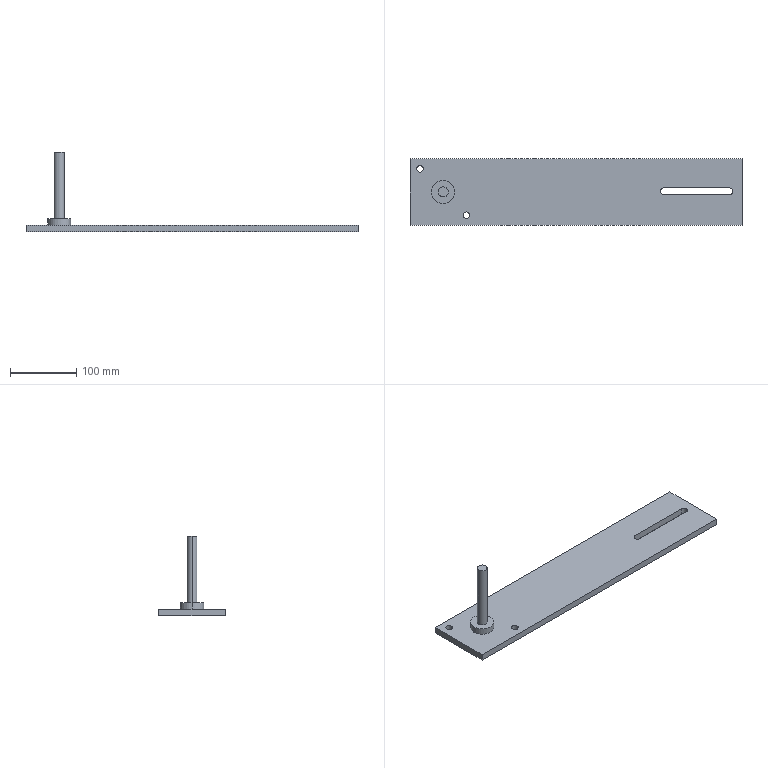Part | SolidWorks | features ICE 5, Extrusion 1 | 1 solid | 24 faces | box 500 x 100 x 120 mm | volume 514971 mm3 | cylinder 12 | plane 12 | commonest cylinder face diameters 9 x4 10 x4 15 x2 35 x2
STEP:
#1=CARTESIAN_POINT('',(-192.5,0.,20.));
#2=VERTEX_POINT('',#1);
#3=CARTESIAN_POINT('',(-207.5,0.,20.));
#4=VERTEX_POINT('',#3);
#5=CARTESIAN_POINT('',(-200.,0.,20.));
#6=DIRECTION('',(0.,0.,1.));
#7=DIRECTION('',(1.,0.,0.));
#8=AXIS2_PLACEMENT_3D('',#5,#6,#7);
#9=CIRCLE('',#8,7.5);
#10=EDGE_CURVE('',#2,#4,#9,.T.);
#11=ORIENTED_EDGE('',*,*,#10,.T.);
#12=CARTESIAN_POINT('',(-207.5,0.,120.));
#13=VERTEX_POINT('',#12);
#14=CARTESIAN_POINT('',(-207.5,0.,20.));
#15=DIRECTION('',(0.,0.,1.));
#16=VECTOR('',#15,1000.);
#17=LINE('',#14,#16);
#18=EDGE_CURVE('',#4,#13,#17,.T.);
#19=ORIENTED_EDGE('',*,*,#18,.T.);
#20=CARTESIAN_POINT('',(-192.5,0.,120.));
#21=VERTEX_POINT('',#20);
#22=CARTESIAN_POINT('',(-200.,0.,120.));
#23=DIRECTION('',(0.,0.,1.));
#24=DIRECTION('',(1.,0.,0.));
#25=AXIS2_PLACEMENT_3D('',#22,#23,#24);
#26=CIRCLE('',#25,7.5);
#27=EDGE_CURVE('',#21,#13,#26,.T.);
#28=ORIENTED_EDGE('',*,*,#27,.F.);
#29=CARTESIAN_POINT('',(-192.5,0.,20.));
#30=DIRECTION('',(0.,0.,1.));
#31=VECTOR('',#30,1000.);
#32=LINE('',#29,#31);
#33=EDGE_CURVE('',#2,#21,#32,.T.);
#34=ORIENTED_EDGE('',*,*,#33,.F.);
#35=EDGE_LOOP('',(#11,#19,#28,#34));
#36=FACE_OUTER_BOUND('',#35,.T.);
#37=CARTESIAN_POINT('',(-200.,0.,20.));
#38=DIRECTION('',(0.,0.,1.));
#39=DIRECTION('',(1.,0.,0.));
#40=AXIS2_PLACEMENT_3D('',#37,#38,#39);
#41=CYLINDRICAL_SURFACE('',#40,7.5);
#42=ADVANCED_FACE('',(#36),#41,.T.);
#43=CARTESIAN_POINT('',(-160.,-35.,0.));
#44=VERTEX_POINT('',#43);
#45=CARTESIAN_POINT('',(-170.,-35.,0.));
#46=VERTEX_POINT('',#45);
#47=CARTESIAN_POINT('',(-165.,-35.,0.));
#48=DIRECTION('',(0.,0.,-1.));
#49=DIRECTION('',(-1.,0.,0.));
#50=AXIS2_PLACEMENT_3D('',#47,#48,#49);
#51=CIRCLE('',#50,5.);
#52=EDGE_CURVE('',#44,#46,#51,.T.);
#53=ORIENTED_EDGE('',*,*,#52,.T.);
#54=CARTESIAN_POINT('',(-170.,-35.,10.));
#55=VERTEX_POINT('',#54);
#56=CARTESIAN_POINT('',(-170.,-35.,-50.));
#57=DIRECTION('',(0.,0.,1.));
#58=VECTOR('',#57,1000.);
#59=LINE('',#56,#58);
#60=EDGE_CURVE('',#46,#55,#59,.T.);
#61=ORIENTED_EDGE('',*,*,#60,.T.);
#62=CARTESIAN_POINT('',(-160.,-35.,10.));
#63=VERTEX_POINT('',#62);
#64=CARTESIAN_POINT('',(-165.,-35.,10.));
#65=DIRECTION('',(0.,0.,1.));
#66=DIRECTION('',(1.,0.,0.));
#67=AXIS2_PLACEMENT_3D('',#64,#65,#66);
#68=CIRCLE('',#67,5.);
#69=EDGE_CURVE('',#55,#63,#68,.T.);
#70=ORIENTED_EDGE('',*,*,#69,.T.);
#71=CARTESIAN_POINT('',(-160.,-35.,-50.));
#72=DIRECTION('',(0.,0.,1.));
#73=VECTOR('',#72,1000.);
#74=LINE('',#71,#73);
#75=EDGE_CURVE('',#44,#63,#74,.T.);
#76=ORIENTED_EDGE('',*,*,#75,.F.);
#77=EDGE_LOOP('',(#53,#61,#70,#76));
#78=FACE_OUTER_BOUND('',#77,.T.);
#79=CARTESIAN_POINT('',(-165.,-35.,-50.));
#80=DIRECTION('',(0.,0.,1.));
#81=DIRECTION('',(1.,0.,0.));
#82=AXIS2_PLACEMENT_3D('',#79,#80,#81);
#83=CYLINDRICAL_SURFACE('',#82,5.);
#84=ADVANCED_FACE('',(#78),#83,.F.);
#85=CARTESIAN_POINT('',(-230.,35.,0.));
#86=VERTEX_POINT('',#85);
#87=CARTESIAN_POINT('',(-240.,35.,0.));
#88=VERTEX_POINT('',#87);
#89=CARTESIAN_POINT('',(-235.,35.,0.));
#90=DIRECTION('',(0.,0.,-1.));
#91=DIRECTION('',(-1.,0.,0.));
#92=AXIS2_PLACEMENT_3D('',#89,#90,#91);
#93=CIRCLE('',#92,5.);
#94=EDGE_CURVE('',#86,#88,#93,.T.);
#95=ORIENTED_EDGE('',*,*,#94,.T.);
#96=CARTESIAN_POINT('',(-240.,35.,10.));
#97=VERTEX_POINT('',#96);
#98=CARTESIAN_POINT('',(-240.,35.,-50.));
#99=DIRECTION('',(0.,0.,1.));
#100=VECTOR('',#99,1000.);
#101=LINE('',#98,#100);
#102=EDGE_CURVE('',#88,#97,#101,.T.);
#103=ORIENTED_EDGE('',*,*,#102,.T.);
#104=CARTESIAN_POINT('',(-230.,35.,10.));
#105=VERTEX_POINT('',#104);
#106=CARTESIAN_POINT('',(-235.,35.,10.));
#107=DIRECTION('',(0.,0.,1.));
#108=DIRECTION('',(1.,0.,0.));
#109=AXIS2_PLACEMENT_3D('',#106,#107,#108);
#110=CIRCLE('',#109,5.);
#111=EDGE_CURVE('',#97,#105,#110,.T.);
#112=ORIENTED_EDGE('',*,*,#111,.T.);
#113=CARTESIAN_POINT('',(-230.,35.,-50.));
#114=DIRECTION('',(0.,0.,1.));
#115=VECTOR('',#114,1000.);
#116=LINE('',#113,#115);
#117=EDGE_CURVE('',#86,#105,#116,.T.);
#118=ORIENTED_EDGE('',*,*,#117,.F.);
#119=EDGE_LOOP('',(#95,#103,#112,#118));
#120=FACE_OUTER_BOUND('',#119,.T.);
#121=CARTESIAN_POINT('',(-235.,35.,-50.));
#122=DIRECTION('',(0.,0.,1.));
#123=DIRECTION('',(1.,0.,0.));
#124=AXIS2_PLACEMENT_3D('',#121,#122,#123);
#125=CYLINDRICAL_SURFACE('',#124,5.);
#126=ADVANCED_FACE('',(#120),#125,.F.);
#127=CARTESIAN_POINT('',(-182.5,0.,20.));
#128=VERTEX_POINT('',#127);
#129=CARTESIAN_POINT('',(-217.5,0.,20.));
#130=VERTEX_POINT('',#129);
#131=CARTESIAN_POINT('',(-200.,0.,20.));
#132=DIRECTION('',(0.,0.,1.));
#133=DIRECTION('',(1.,0.,0.));
#134=AXIS2_PLACEMENT_3D('',#131,#132,#133);
#135=CIRCLE('',#134,17.5);
#136=EDGE_CURVE('',#128,#130,#135,.T.);
#137=ORIENTED_EDGE('',*,*,#136,.F.);
#138=CARTESIAN_POINT('',(-182.5,0.,10.));
#139=VERTEX_POINT('',#138);
#140=CARTESIAN_POINT('',(-182.5,0.,70.));
#141=DIRECTION('',(0.,0.,-1.));
#142=VECTOR('',#141,1000.);
#143=LINE('',#140,#142);
#144=EDGE_CURVE('',#128,#139,#143,.T.);
#145=ORIENTED_EDGE('',*,*,#144,.T.);
#146=CARTESIAN_POINT('',(-217.5,0.,10.));
#147=VERTEX_POINT('',#146);
#148=CARTESIAN_POINT('',(-200.,0.,10.));
#149=DIRECTION('',(0.,0.,1.));
#150=DIRECTION('',(-1.,0.,0.));
#151=AXIS2_PLACEMENT_3D('',#148,#149,#150);
#152=CIRCLE('',#151,17.5);
#153=EDGE_CURVE('',#139,#147,#152,.T.);
#154=ORIENTED_EDGE('',*,*,#153,.T.);
#155=CARTESIAN_POINT('',(-217.5,0.,70.));
#156=DIRECTION('',(0.,0.,-1.));
#157=VECTOR('',#156,1000.);
#158=LINE('',#155,#157);
#159=EDGE_CURVE('',#130,#147,#158,.T.);
#160=ORIENTED_EDGE('',*,*,#159,.F.);
#161=EDGE_LOOP('',(#137,#145,#154,#160));
#162=FACE_OUTER_BOUND('',#161,.T.);
#163=CARTESIAN_POINT('',(-200.,0.,70.));
#164=DIRECTION('',(0.,0.,-1.));
#165=DIRECTION('',(-1.,0.,0.));
#166=AXIS2_PLACEMENT_3D('',#163,#164,#165);
#167=CYLINDRICAL_SURFACE('',#166,17.5);
#168=ADVANCED_FACE('',(#162),#167,.T.);
#169=ORIENTED_EDGE('',*,*,#144,.F.);
#170=CARTESIAN_POINT('',(-200.,0.,20.));
#171=DIRECTION('',(0.,0.,1.));
#172=DIRECTION('',(1.,0.,0.));
#173=AXIS2_PLACEMENT_3D('',#170,#171,#172);
#174=CIRCLE('',#173,17.5);
#175=EDGE_CURVE('',#130,#128,#174,.T.);
#176=ORIENTED_EDGE('',*,*,#175,.F.);
#177=ORIENTED_EDGE('',*,*,#159,.T.);
#178=CARTESIAN_POINT('',(-200.,0.,10.));
#179=DIRECTION('',(0.,0.,1.));
#180=DIRECTION('',(-1.,0.,0.));
#181=AXIS2_PLACEMENT_3D('',#178,#179,#180);
#182=CIRCLE('',#181,17.5);
#183=EDGE_CURVE('',#147,#139,#182,.T.);
#184=ORIENTED_EDGE('',*,*,#183,.T.);
#185=EDGE_LOOP('',(#169,#176,#177,#184));
#186=FACE_OUTER_BOUND('',#185,.T.);
#187=CARTESIAN_POINT('',(-200.,0.,70.));
#188=DIRECTION('',(0.,0.,-1.));
#189=DIRECTION('',(-1.,0.,0.));
#190=AXIS2_PLACEMENT_3D('',#187,#188,#189);
#191=CYLINDRICAL_SURFACE('',#190,17.5);
#192=ADVANCED_FACE('',(#186),#191,.T.);
#193=CARTESIAN_POINT('',(-250.,50.,10.));
#194=VERTEX_POINT('',#193);
#195=CARTESIAN_POINT('',(-250.,-50.,10.));
#196=VERTEX_POINT('',#195);
#197=CARTESIAN_POINT('',(-250.,50.,10.));
#198=DIRECTION('',(0.,-1.,0.));
#199=VECTOR('',#198,1000.);
#200=LINE('',#197,#199);
#201=EDGE_CURVE('',#194,#196,#200,.T.);
#202=ORIENTED_EDGE('',*,*,#201,.T.);
#203=CARTESIAN_POINT('',(250.,-50.,10.));
#204=VERTEX_POINT('',#203);
#205=CARTESIAN_POINT('',(250.,-50.,10.));
#206=DIRECTION('',(1.,0.,0.));
#207=VECTOR('',#206,1000.);
#208=LINE('',#205,#207);
#209=EDGE_CURVE('',#196,#204,#208,.T.);
#210=ORIENTED_EDGE('',*,*,#209,.T.);
#211=CARTESIAN_POINT('',(250.,50.,10.));
#212=VERTEX_POINT('',#211);
#213=CARTESIAN_POINT('',(250.,50.,10.));
#214=DIRECTION('',(0.,1.,0.));
#215=VECTOR('',#214,1000.);
#216=LINE('',#213,#215);
#217=EDGE_CURVE('',#204,#212,#216,.T.);
#218=ORIENTED_EDGE('',*,*,#217,.T.);
#219=CARTESIAN_POINT('',(250.,50.,10.));
#220=DIRECTION('',(-1.,0.,0.));
#221=VECTOR('',#220,1000.);
#222=LINE('',#219,#221);
#223=EDGE_CURVE('',#212,#194,#222,.T.);
#224=ORIENTED_EDGE('',*,*,#223,.T.);
#225=EDGE_LOOP('',(#202,#210,#218,#224));
#226=FACE_OUTER_BOUND('',#225,.T.);
#227=CARTESIAN_POINT('',(231.805,6.068,10.));
#228=VERTEX_POINT('',#227);
#229=CARTESIAN_POINT('',(131.558,6.068,10.));
#230=VERTEX_POINT('',#229);
#231=CARTESIAN_POINT('',(231.805,6.068,10.));
#232=DIRECTION('',(-1.,0.,0.));
#233=VECTOR('',#232,1000.);
#234=LINE('',#231,#233);
#235=EDGE_CURVE('',#228,#230,#234,.T.);
#236=ORIENTED_EDGE('',*,*,#235,.F.);
#237=CARTESIAN_POINT('',(236.305,1.568,10.));
#238=VERTEX_POINT('',#237);
#239=CARTESIAN_POINT('',(231.805,1.568,10.));
#240=DIRECTION('',(0.,0.,1.));
#241=DIRECTION('',(1.,0.,0.));
#242=AXIS2_PLACEMENT_3D('',#239,#240,#241);
#243=CIRCLE('',#242,4.5);
#244=EDGE_CURVE('',#238,#228,#243,.T.);
#245=ORIENTED_EDGE('',*,*,#244,.F.);
#246=CARTESIAN_POINT('',(236.305,0.5678,10.));
#247=VERTEX_POINT('',#246);
#248=CARTESIAN_POINT('',(236.305,0.5678,10.));
#249=DIRECTION('',(0.,1.,0.));
#250=VECTOR('',#249,1000.);
#251=LINE('',#248,#250);
#252=EDGE_CURVE('',#247,#238,#251,.T.);
#253=ORIENTED_EDGE('',*,*,#252,.F.);
#254=CARTESIAN_POINT('',(231.805,-3.932,10.));
#255=VERTEX_POINT('',#254);
#256=CARTESIAN_POINT('',(231.805,0.5678,10.));
#257=DIRECTION('',(0.,0.,1.));
#258=DIRECTION('',(1.,0.,0.));
#259=AXIS2_PLACEMENT_3D('',#256,#257,#258);
#260=CIRCLE('',#259,4.5);
#261=EDGE_CURVE('',#255,#247,#260,.T.);
#262=ORIENTED_EDGE('',*,*,#261,.F.);
#263=CARTESIAN_POINT('',(131.558,-3.932,10.));
#264=VERTEX_POINT('',#263);
#265=CARTESIAN_POINT('',(231.805,-3.932,10.));
#266=DIRECTION('',(1.,0.,0.));
#267=VECTOR('',#266,1000.);
#268=LINE('',#265,#267);
#269=EDGE_CURVE('',#264,#255,#268,.T.);
#270=ORIENTED_EDGE('',*,*,#269,.F.);
#271=CARTESIAN_POINT('',(127.058,0.5678,10.));
#272=VERTEX_POINT('',#271);
#273=CARTESIAN_POINT('',(131.558,0.5678,10.));
#274=DIRECTION('',(0.,0.,1.));
#275=DIRECTION('',(-1.,0.,0.));
#276=AXIS2_PLACEMENT_3D('',#273,#274,#275);
#277=CIRCLE('',#276,4.5);
#278=EDGE_CURVE('',#272,#264,#277,.T.);
#279=ORIENTED_EDGE('',*,*,#278,.F.);
#280=CARTESIAN_POINT('',(127.058,1.568,10.));
#281=VERTEX_POINT('',#280);
#282=CARTESIAN_POINT('',(127.058,0.5678,10.));
#283=DIRECTION('',(0.,-1.,0.));
#284=VECTOR('',#283,1000.);
#285=LINE('',#282,#284);
#286=EDGE_CURVE('',#281,#272,#285,.T.);
#287=ORIENTED_EDGE('',*,*,#286,.F.);
#288=CARTESIAN_POINT('',(131.558,1.568,10.));
#289=DIRECTION('',(0.,0.,1.));
#290=DIRECTION('',(-1.,0.,0.));
#291=AXIS2_PLACEMENT_3D('',#288,#289,#290);
#292=CIRCLE('',#291,4.5);
#293=EDGE_CURVE('',#230,#281,#292,.T.);
#294=ORIENTED_EDGE('',*,*,#293,.F.);
#295=EDGE_LOOP('',(#236,#245,#253,#262,#270,#279,#287,#294));
#296=FACE_BOUND('',#295,.T.);
#297=CARTESIAN_POINT('',(-235.,35.,10.));
#298=DIRECTION('',(0.,0.,1.));
#299=DIRECTION('',(1.,0.,0.));
#300=AXIS2_PLACEMENT_3D('',#297,#298,#299);
#301=CIRCLE('',#300,5.);
#302=EDGE_CURVE('',#105,#97,#301,.T.);
#303=ORIENTED_EDGE('',*,*,#302,.F.);
#304=ORIENTED_EDGE('',*,*,#111,.F.);
#305=EDGE_LOOP('',(#303,#304));
#306=FACE_BOUND('',#305,.T.);
#307=CARTESIAN_POINT('',(-165.,-35.,10.));
#308=DIRECTION('',(0.,0.,1.));
#309=DIRECTION('',(1.,0.,0.));
#310=AXIS2_PLACEMENT_3D('',#307,#308,#309);
#311=CIRCLE('',#310,5.);
#312=EDGE_CURVE('',#63,#55,#311,.T.);
#313=ORIENTED_EDGE('',*,*,#312,.F.);
#314=ORIENTED_EDGE('',*,*,#69,.F.);
#315=EDGE_LOOP('',(#313,#314));
#316=FACE_BOUND('',#315,.T.);
#317=ORIENTED_EDGE('',*,*,#183,.F.);
#318=ORIENTED_EDGE('',*,*,#153,.F.);
#319=EDGE_LOOP('',(#317,#318));
#320=FACE_BOUND('',#319,.T.);
#321=CARTESIAN_POINT('',(-250.,-50.,10.));
#322=DIRECTION('',(0.,0.,-1.));
#323=DIRECTION('',(-1.,0.,0.));
#324=AXIS2_PLACEMENT_3D('',#321,#322,#323);
#325=PLANE('',#324);
#326=ADVANCED_FACE('',(#226,#296,#306,#316,#320),#325,.F.);
#327=CARTESIAN_POINT('',(-250.,50.,0.));
#328=VERTEX_POINT('',#327);
#329=CARTESIAN_POINT('',(-250.,-50.,0.));
#330=VERTEX_POINT('',#329);
#331=CARTESIAN_POINT('',(-250.,50.,0.));
#332=DIRECTION('',(0.,-1.,0.));
#333=VECTOR('',#332,1000.);
#334=LINE('',#331,#333);
#335=EDGE_CURVE('',#328,#330,#334,.T.);
#336=ORIENTED_EDGE('',*,*,#335,.T.);
#337=CARTESIAN_POINT('',(-250.,-50.,10.));
#338=DIRECTION('',(0.,0.,-1.));
#339=VECTOR('',#338,1000.);
#340=LINE('',#337,#339);
#341=EDGE_CURVE('',#196,#330,#340,.T.);
#342=ORIENTED_EDGE('',*,*,#341,.F.);
#343=ORIENTED_EDGE('',*,*,#201,.F.);
#344=CARTESIAN_POINT('',(-250.,50.,10.));
#345=DIRECTION('',(0.,0.,-1.));
#346=VECTOR('',#345,1000.);
#347=LINE('',#344,#346);
#348=EDGE_CURVE('',#194,#328,#347,.T.);
#349=ORIENTED_EDGE('',*,*,#348,.T.);
#350=EDGE_LOOP('',(#336,#342,#343,#349));
#351=FACE_OUTER_BOUND('',#350,.T.);
#352=CARTESIAN_POINT('',(-250.,50.,10.));
#353=DIRECTION('',(1.,0.,0.));
#354=DIRECTION('',(0.,0.,-1.));
#355=AXIS2_PLACEMENT_3D('',#352,#353,#354);
#356=PLANE('',#355);
#357=ADVANCED_FACE('',(#351),#356,.F.);
#358=CARTESIAN_POINT('',(250.,-50.,0.));
#359=VERTEX_POINT('',#358);
#360=CARTESIAN_POINT('',(250.,-50.,0.));
#361=DIRECTION('',(1.,0.,0.));
#362=VECTOR('',#361,1000.);
#363=LINE('',#360,#362);
#364=EDGE_CURVE('',#330,#359,#363,.T.);
#365=ORIENTED_EDGE('',*,*,#364,.T.);
#366=CARTESIAN_POINT('',(250.,-50.,10.));
#367=DIRECTION('',(0.,0.,-1.));
#368=VECTOR('',#367,1000.);
#369=LINE('',#366,#368);
#370=EDGE_CURVE('',#204,#359,#369,.T.);
#371=ORIENTED_EDGE('',*,*,#370,.F.);
#372=ORIENTED_EDGE('',*,*,#209,.F.);
#373=ORIENTED_EDGE('',*,*,#341,.T.);
#374=EDGE_LOOP('',(#365,#371,#372,#373));
#375=FACE_OUTER_BOUND('',#374,.T.);
#376=CARTESIAN_POINT('',(250.,-50.,10.));
#377=DIRECTION('',(0.,1.,0.));
#378=DIRECTION('',(-1.,0.,0.));
#379=AXIS2_PLACEMENT_3D('',#376,#377,#378);
#380=PLANE('',#379);
#381=ADVANCED_FACE('',(#375),#380,.F.);
#382=CARTESIAN_POINT('',(250.,50.,0.));
#383=VERTEX_POINT('',#382);
#384=CARTESIAN_POINT('',(250.,50.,0.));
#385=DIRECTION('',(0.,1.,0.));
#386=VECTOR('',#385,1000.);
#387=LINE('',#384,#386);
#388=EDGE_CURVE('',#359,#383,#387,.T.);
#389=ORIENTED_EDGE('',*,*,#388,.T.);
#390=CARTESIAN_POINT('',(250.,50.,10.));
#391=DIRECTION('',(0.,0.,-1.));
#392=VECTOR('',#391,1000.);
#393=LINE('',#390,#392);
#394=EDGE_CURVE('',#212,#383,#393,.T.);
#395=ORIENTED_EDGE('',*,*,#394,.F.);
#396=ORIENTED_EDGE('',*,*,#217,.F.);
#397=ORIENTED_EDGE('',*,*,#370,.T.);
#398=EDGE_LOOP('',(#389,#395,#396,#397));
#399=FACE_OUTER_BOUND('',#398,.T.);
#400=CARTESIAN_POINT('',(250.,50.,10.));
#401=DIRECTION('',(-1.,0.,0.));
#402=DIRECTION('',(0.,0.,1.));
#403=AXIS2_PLACEMENT_3D('',#400,#401,#402);
#404=PLANE('',#403);
#405=ADVANCED_FACE('',(#399),#404,.F.);
#406=CARTESIAN_POINT('',(250.,50.,0.));
#407=DIRECTION('',(-1.,0.,0.));
#408=VECTOR('',#407,1000.);
#409=LINE('',#406,#408);
#410=EDGE_CURVE('',#383,#328,#409,.T.);
#411=ORIENTED_EDGE('',*,*,#410,.T.);
#412=ORIENTED_EDGE('',*,*,#348,.F.);
#413=ORIENTED_EDGE('',*,*,#223,.F.);
#414=ORIENTED_EDGE('',*,*,#394,.T.);
#415=EDGE_LOOP('',(#411,#412,#413,#414));
#416=FACE_OUTER_BOUND('',#415,.T.);
#417=CARTESIAN_POINT('',(250.,50.,10.));
#418=DIRECTION('',(0.,-1.,0.));
#419=DIRECTION('',(1.,0.,0.));
#420=AXIS2_PLACEMENT_3D('',#417,#418,#419);
#421=PLANE('',#420);
#422=ADVANCED_FACE('',(#416),#421,.F.);
#423=ORIENTED_EDGE('',*,*,#52,.F.);
#424=CARTESIAN_POINT('',(-165.,-35.,0.));
#425=DIRECTION('',(0.,0.,-1.));
#426=DIRECTION('',(-1.,0.,0.));
#427=AXIS2_PLACEMENT_3D('',#424,#425,#426);
#428=CIRCLE('',#427,5.);
#429=EDGE_CURVE('',#46,#44,#428,.T.);
#430=ORIENTED_EDGE('',*,*,#429,.F.);
#431=EDGE_LOOP('',(#423,#430));
#432=FACE_BOUND('',#431,.T.);
#433=ORIENTED_EDGE('',*,*,#94,.F.);
#434=CARTESIAN_POINT('',(-235.,35.,0.));
#435=DIRECTION('',(0.,0.,-1.));
#436=DIRECTION('',(-1.,0.,0.));
#437=AXIS2_PLACEMENT_3D('',#434,#435,#436);
#438=CIRCLE('',#437,5.);
#439=EDGE_CURVE('',#88,#86,#438,.T.);
#440=ORIENTED_EDGE('',*,*,#439,.F.);
#441=EDGE_LOOP('',(#433,#440));
#442=FACE_BOUND('',#441,.T.);
#443=CARTESIAN_POINT('',(231.805,6.068,0.));
#444=VERTEX_POINT('',#443);
#445=CARTESIAN_POINT('',(236.305,1.568,0.));
#446=VERTEX_POINT('',#445);
#447=CARTESIAN_POINT('',(231.805,1.568,0.));
#448=DIRECTION('',(0.,0.,-1.));
#449=DIRECTION('',(-1.,0.,0.));
#450=AXIS2_PLACEMENT_3D('',#447,#448,#449);
#451=CIRCLE('',#450,4.5);
#452=EDGE_CURVE('',#444,#446,#451,.T.);
#453=ORIENTED_EDGE('',*,*,#452,.F.);
#454=CARTESIAN_POINT('',(131.558,6.068,0.));
#455=VERTEX_POINT('',#454);
#456=CARTESIAN_POINT('',(-250.,6.068,0.));
#457=DIRECTION('',(1.,0.,0.));
#458=VECTOR('',#457,1000.);
#459=LINE('',#456,#458);
#460=EDGE_CURVE('',#455,#444,#459,.T.);
#461=ORIENTED_EDGE('',*,*,#460,.F.);
#462=CARTESIAN_POINT('',(127.058,1.568,0.));
#463=VERTEX_POINT('',#462);
#464=CARTESIAN_POINT('',(131.558,1.568,0.));
#465=DIRECTION('',(0.,0.,-1.));
#466=DIRECTION('',(-1.,0.,0.));
#467=AXIS2_PLACEMENT_3D('',#464,#465,#466);
#468=CIRCLE('',#467,4.5);
#469=EDGE_CURVE('',#463,#455,#468,.T.);
#470=ORIENTED_EDGE('',*,*,#469,.F.);
#471=CARTESIAN_POINT('',(127.058,0.5678,0.));
#472=VERTEX_POINT('',#471);
#473=CARTESIAN_POINT('',(127.058,-50.,0.));
#474=DIRECTION('',(0.,1.,0.));
#475=VECTOR('',#474,1000.);
#476=LINE('',#473,#475);
#477=EDGE_CURVE('',#472,#463,#476,.T.);
#478=ORIENTED_EDGE('',*,*,#477,.F.);
#479=CARTESIAN_POINT('',(131.558,-3.932,0.));
#480=VERTEX_POINT('',#479);
#481=CARTESIAN_POINT('',(131.558,0.5678,0.));
#482=DIRECTION('',(0.,0.,-1.));
#483=DIRECTION('',(-1.,0.,0.));
#484=AXIS2_PLACEMENT_3D('',#481,#482,#483);
#485=CIRCLE('',#484,4.5);
#486=EDGE_CURVE('',#480,#472,#485,.T.);
#487=ORIENTED_EDGE('',*,*,#486,.F.);
#488=CARTESIAN_POINT('',(231.805,-3.932,0.));
#489=VERTEX_POINT('',#488);
#490=CARTESIAN_POINT('',(-250.,-3.932,0.));
#491=DIRECTION('',(-1.,0.,0.));
#492=VECTOR('',#491,1000.);
#493=LINE('',#490,#492);
#494=EDGE_CURVE('',#489,#480,#493,.T.);
#495=ORIENTED_EDGE('',*,*,#494,.F.);
#496=CARTESIAN_POINT('',(236.305,0.5678,0.));
#497=VERTEX_POINT('',#496);
#498=CARTESIAN_POINT('',(231.805,0.5678,0.));
#499=DIRECTION('',(0.,0.,-1.));
#500=DIRECTION('',(-1.,0.,0.));
#501=AXIS2_PLACEMENT_3D('',#498,#499,#500);
#502=CIRCLE('',#501,4.5);
#503=EDGE_CURVE('',#497,#489,#502,.T.);
#504=ORIENTED_EDGE('',*,*,#503,.F.);
#505=CARTESIAN_POINT('',(236.305,-50.,0.));
#506=DIRECTION('',(0.,-1.,0.));
#507=VECTOR('',#506,1000.);
#508=LINE('',#505,#507);
#509=EDGE_CURVE('',#446,#497,#508,.T.);
#510=ORIENTED_EDGE('',*,*,#509,.F.);
#511=EDGE_LOOP('',(#453,#461,#470,#478,#487,#495,#504,#510));
#512=FACE_BOUND('',#511,.T.);
#513=ORIENTED_EDGE('',*,*,#335,.F.);
#514=ORIENTED_EDGE('',*,*,#410,.F.);
#515=ORIENTED_EDGE('',*,*,#388,.F.);
#516=ORIENTED_EDGE('',*,*,#364,.F.);
#517=EDGE_LOOP('',(#513,#514,#515,#516));
#518=FACE_OUTER_BOUND('',#517,.T.);
#519=CARTESIAN_POINT('',(-250.,-50.,0.));
#520=DIRECTION('',(0.,0.,-1.));
#521=DIRECTION('',(-1.,0.,0.));
#522=AXIS2_PLACEMENT_3D('',#519,#520,#521);
#523=PLANE('',#522);
#524=ADVANCED_FACE('',(#432,#442,#512,#518),#523,.T.);
#525=ORIENTED_EDGE('',*,*,#452,.T.);
#526=CARTESIAN_POINT('',(236.305,1.568,-50.));
#527=DIRECTION('',(0.,0.,1.));
#528=VECTOR('',#527,1000.);
#529=LINE('',#526,#528);
#530=EDGE_CURVE('',#446,#238,#529,.T.);
#531=ORIENTED_EDGE('',*,*,#530,.T.);
#532=ORIENTED_EDGE('',*,*,#244,.T.);
#533=CARTESIAN_POINT('',(231.805,6.068,-50.));
#534=DIRECTION('',(0.,0.,1.));
#535=VECTOR('',#534,1000.);
#536=LINE('',#533,#535);
#537=EDGE_CURVE('',#444,#228,#536,.T.);
#538=ORIENTED_EDGE('',*,*,#537,.F.);
#539=EDGE_LOOP('',(#525,#531,#532,#538));
#540=FACE_OUTER_BOUND('',#539,.T.);
#541=CARTESIAN_POINT('',(231.805,1.568,-50.));
#542=DIRECTION('',(0.,0.,1.));
#543=DIRECTION('',(1.,0.,0.));
#544=AXIS2_PLACEMENT_3D('',#541,#542,#543);
#545=CYLINDRICAL_SURFACE('',#544,4.5);
#546=ADVANCED_FACE('',(#540),#545,.F.);
#547=ORIENTED_EDGE('',*,*,#509,.T.);
#548=CARTESIAN_POINT('',(236.305,0.5678,-50.));
#549=DIRECTION('',(0.,0.,1.));
#550=VECTOR('',#549,1000.);
#551=LINE('',#548,#550);
#552=EDGE_CURVE('',#497,#247,#551,.T.);
#553=ORIENTED_EDGE('',*,*,#552,.T.);
#554=ORIENTED_EDGE('',*,*,#252,.T.);
#555=ORIENTED_EDGE('',*,*,#530,.F.);
#556=EDGE_LOOP('',(#547,#553,#554,#555));
#557=FACE_OUTER_BOUND('',#556,.T.);
#558=CARTESIAN_POINT('',(236.305,0.5678,-50.));
#559=DIRECTION('',(1.,0.,0.));
#560=DIRECTION('',(0.,0.,-1.));
#561=AXIS2_PLACEMENT_3D('',#558,#559,#560);
#562=PLANE('',#561);
#563=ADVANCED_FACE('',(#557),#562,.F.);
#564=ORIENTED_EDGE('',*,*,#503,.T.);
#565=CARTESIAN_POINT('',(231.805,-3.932,-50.));
#566=DIRECTION('',(0.,0.,1.));
#567=VECTOR('',#566,1000.);
#568=LINE('',#565,#567);
#569=EDGE_CURVE('',#489,#255,#568,.T.);
#570=ORIENTED_EDGE('',*,*,#569,.T.);
#571=ORIENTED_EDGE('',*,*,#261,.T.);
#572=ORIENTED_EDGE('',*,*,#552,.F.);
#573=EDGE_LOOP('',(#564,#570,#571,#572));
#574=FACE_OUTER_BOUND('',#573,.T.);
#575=CARTESIAN_POINT('',(231.805,0.5678,-50.));
#576=DIRECTION('',(0.,0.,1.));
#577=DIRECTION('',(1.,0.,0.));
#578=AXIS2_PLACEMENT_3D('',#575,#576,#577);
#579=CYLINDRICAL_SURFACE('',#578,4.5);
#580=ADVANCED_FACE('',(#574),#579,.F.);
#581=ORIENTED_EDGE('',*,*,#494,.T.);
#582=CARTESIAN_POINT('',(131.558,-3.932,-50.));
#583=DIRECTION('',(0.,0.,1.));
#584=VECTOR('',#583,1000.);
#585=LINE('',#582,#584);
#586=EDGE_CURVE('',#480,#264,#585,.T.);
#587=ORIENTED_EDGE('',*,*,#586,.T.);
#588=ORIENTED_EDGE('',*,*,#269,.T.);
#589=ORIENTED_EDGE('',*,*,#569,.F.);
#590=EDGE_LOOP('',(#581,#587,#588,#589));
#591=FACE_OUTER_BOUND('',#590,.T.);
#592=CARTESIAN_POINT('',(231.805,-3.932,-50.));
#593=DIRECTION('',(0.,-1.,0.));
#594=DIRECTION('',(1.,0.,0.));
#595=AXIS2_PLACEMENT_3D('',#592,#593,#594);
#596=PLANE('',#595);
#597=ADVANCED_FACE('',(#591),#596,.F.);
#598=ORIENTED_EDGE('',*,*,#486,.T.);
#599=CARTESIAN_POINT('',(127.058,0.5678,-50.));
#600=DIRECTION('',(0.,0.,1.));
#601=VECTOR('',#600,1000.);
#602=LINE('',#599,#601);
#603=EDGE_CURVE('',#472,#272,#602,.T.);
#604=ORIENTED_EDGE('',*,*,#603,.T.);
#605=ORIENTED_EDGE('',*,*,#278,.T.);
#606=ORIENTED_EDGE('',*,*,#586,.F.);
#607=EDGE_LOOP('',(#598,#604,#605,#606));
#608=FACE_OUTER_BOUND('',#607,.T.);
#609=CARTESIAN_POINT('',(131.558,0.5678,-50.));
#610=DIRECTION('',(0.,0.,1.));
#611=DIRECTION('',(1.,0.,0.));
#612=AXIS2_PLACEMENT_3D('',#609,#610,#611);
#613=CYLINDRICAL_SURFACE('',#612,4.5);
#614=ADVANCED_FACE('',(#608),#613,.F.);
#615=ORIENTED_EDGE('',*,*,#477,.T.);
#616=CARTESIAN_POINT('',(127.058,1.568,-50.));
#617=DIRECTION('',(0.,0.,1.));
#618=VECTOR('',#617,1000.);
#619=LINE('',#616,#618);
#620=EDGE_CURVE('',#463,#281,#619,.T.);
#621=ORIENTED_EDGE('',*,*,#620,.T.);
#622=ORIENTED_EDGE('',*,*,#286,.T.);
#623=ORIENTED_EDGE('',*,*,#603,.F.);
#624=EDGE_LOOP('',(#615,#621,#622,#623));
#625=FACE_OUTER_BOUND('',#624,.T.);
#626=CARTESIAN_POINT('',(127.058,0.5678,-50.));
#627=DIRECTION('',(-1.,0.,0.));
#628=DIRECTION('',(0.,0.,1.));
#629=AXIS2_PLACEMENT_3D('',#626,#627,#628);
#630=PLANE('',#629);
#631=ADVANCED_FACE('',(#625),#630,.F.);
#632=ORIENTED_EDGE('',*,*,#469,.T.);
#633=CARTESIAN_POINT('',(131.558,6.068,-50.));
#634=DIRECTION('',(0.,0.,1.));
#635=VECTOR('',#634,1000.);
#636=LINE('',#633,#635);
#637=EDGE_CURVE('',#455,#230,#636,.T.);
#638=ORIENTED_EDGE('',*,*,#637,.T.);
#639=ORIENTED_EDGE('',*,*,#293,.T.);
#640=ORIENTED_EDGE('',*,*,#620,.F.);
#641=EDGE_LOOP('',(#632,#638,#639,#640));
#642=FACE_OUTER_BOUND('',#641,.T.);
#643=CARTESIAN_POINT('',(131.558,1.568,-50.));
#644=DIRECTION('',(0.,0.,1.));
#645=DIRECTION('',(1.,0.,0.));
#646=AXIS2_PLACEMENT_3D('',#643,#644,#645);
#647=CYLINDRICAL_SURFACE('',#646,4.5);
#648=ADVANCED_FACE('',(#642),#647,.F.);
#649=ORIENTED_EDGE('',*,*,#460,.T.);
#650=ORIENTED_EDGE('',*,*,#537,.T.);
#651=ORIENTED_EDGE('',*,*,#235,.T.);
#652=ORIENTED_EDGE('',*,*,#637,.F.);
#653=EDGE_LOOP('',(#649,#650,#651,#652));
#654=FACE_OUTER_BOUND('',#653,.T.);
#655=CARTESIAN_POINT('',(231.805,6.068,-50.));
#656=DIRECTION('',(0.,1.,0.));
#657=DIRECTION('',(-1.,0.,0.));
#658=AXIS2_PLACEMENT_3D('',#655,#656,#657);
#659=PLANE('',#658);
#660=ADVANCED_FACE('',(#654),#659,.F.);
#661=ORIENTED_EDGE('',*,*,#102,.F.);
#662=ORIENTED_EDGE('',*,*,#439,.T.);
#663=ORIENTED_EDGE('',*,*,#117,.T.);
#664=ORIENTED_EDGE('',*,*,#302,.T.);
#665=EDGE_LOOP('',(#661,#662,#663,#664));
#666=FACE_OUTER_BOUND('',#665,.T.);
#667=CARTESIAN_POINT('',(-235.,35.,-50.));
#668=DIRECTION('',(0.,0.,1.));
#669=DIRECTION('',(1.,0.,0.));
#670=AXIS2_PLACEMENT_3D('',#667,#668,#669);
#671=CYLINDRICAL_SURFACE('',#670,5.);
#672=ADVANCED_FACE('',(#666),#671,.F.);
#673=ORIENTED_EDGE('',*,*,#60,.F.);
#674=ORIENTED_EDGE('',*,*,#429,.T.);
#675=ORIENTED_EDGE('',*,*,#75,.T.);
#676=ORIENTED_EDGE('',*,*,#312,.T.);
#677=EDGE_LOOP('',(#673,#674,#675,#676));
#678=FACE_OUTER_BOUND('',#677,.T.);
#679=CARTESIAN_POINT('',(-165.,-35.,-50.));
#680=DIRECTION('',(0.,0.,1.));
#681=DIRECTION('',(1.,0.,0.));
#682=AXIS2_PLACEMENT_3D('',#679,#680,#681);
#683=CYLINDRICAL_SURFACE('',#682,5.);
#684=ADVANCED_FACE('',(#678),#683,.F.);
#685=ORIENTED_EDGE('',*,*,#10,.F.);
#686=CARTESIAN_POINT('',(-200.,0.,20.));
#687=DIRECTION('',(0.,0.,1.));
#688=DIRECTION('',(1.,0.,0.));
#689=AXIS2_PLACEMENT_3D('',#686,#687,#688);
#690=CIRCLE('',#689,7.5);
#691=EDGE_CURVE('',#4,#2,#690,.T.);
#692=ORIENTED_EDGE('',*,*,#691,.F.);
#693=EDGE_LOOP('',(#685,#692));
#694=FACE_BOUND('',#693,.T.);
#695=ORIENTED_EDGE('',*,*,#175,.T.);
#696=ORIENTED_EDGE('',*,*,#136,.T.);
#697=EDGE_LOOP('',(#695,#696));
#698=FACE_OUTER_BOUND('',#697,.T.);
#699=CARTESIAN_POINT('',(-200.,0.,20.));
#700=DIRECTION('',(0.,0.,1.));
#701=DIRECTION('',(1.,0.,0.));
#702=AXIS2_PLACEMENT_3D('',#699,#700,#701);
#703=PLANE('',#702);
#704=ADVANCED_FACE('',(#694,#698),#703,.T.);
#705=ORIENTED_EDGE('',*,*,#18,.F.);
#706=ORIENTED_EDGE('',*,*,#691,.T.);
#707=ORIENTED_EDGE('',*,*,#33,.T.);
#708=CARTESIAN_POINT('',(-200.,0.,120.));
#709=DIRECTION('',(0.,0.,1.));
#710=DIRECTION('',(1.,0.,0.));
#711=AXIS2_PLACEMENT_3D('',#708,#709,#710);
#712=CIRCLE('',#711,7.5);
#713=EDGE_CURVE('',#13,#21,#712,.T.);
#714=ORIENTED_EDGE('',*,*,#713,.F.);
#715=EDGE_LOOP('',(#705,#706,#707,#714));
#716=FACE_OUTER_BOUND('',#715,.T.);
#717=CARTESIAN_POINT('',(-200.,0.,20.));
#718=DIRECTION('',(0.,0.,1.));
#719=DIRECTION('',(1.,0.,0.));
#720=AXIS2_PLACEMENT_3D('',#717,#718,#719);
#721=CYLINDRICAL_SURFACE('',#720,7.5);
#722=ADVANCED_FACE('',(#716),#721,.T.);
#723=ORIENTED_EDGE('',*,*,#27,.T.);
#724=ORIENTED_EDGE('',*,*,#713,.T.);
#725=EDGE_LOOP('',(#723,#724));
#726=FACE_OUTER_BOUND('',#725,.T.);
#727=CARTESIAN_POINT('',(-200.,0.,120.));
#728=DIRECTION('',(0.,0.,1.));
#729=DIRECTION('',(1.,0.,0.));
#730=AXIS2_PLACEMENT_3D('',#727,#728,#729);
#731=PLANE('',#730);
#732=ADVANCED_FACE('',(#726),#731,.T.);
#733=CLOSED_SHELL('',(#42,#84,#126,#168,#192,#326,#357,#381,#405,#422,#524,#546,#563,#580,#597,#614,#631,#648,#660,#672,#684,#704,#722,#732));
#734=MANIFOLD_SOLID_BREP('',#733);
#735=CARTESIAN_POINT('',(0.,0.,0.));
#736=DIRECTION('',(0.,0.,1.));
#737=DIRECTION('',(1.,0.,0.));
#738=AXIS2_PLACEMENT_3D('',#735,#736,#737);
#739=(LENGTH_UNIT()NAMED_UNIT(*)SI_UNIT(.MILLI.,.METRE.));
#740=UNCERTAINTY_MEASURE_WITH_UNIT(LENGTH_MEASURE(0.00001),#739,'','');
#741=(NAMED_UNIT(*)PLANE_ANGLE_UNIT()SI_UNIT($,.RADIAN.));
#742=(NAMED_UNIT(*)SI_UNIT($,.STERADIAN.)SOLID_ANGLE_UNIT());
#743=(GEOMETRIC_REPRESENTATION_CONTEXT(3)GLOBAL_UNCERTAINTY_ASSIGNED_CONTEXT((#740))GLOBAL_UNIT_ASSIGNED_CONTEXT((#739,#741,#742))REPRESENTATION_CONTEXT('',''));
#744=ADVANCED_BREP_SHAPE_REPRESENTATION('',(#734,#738),#743);